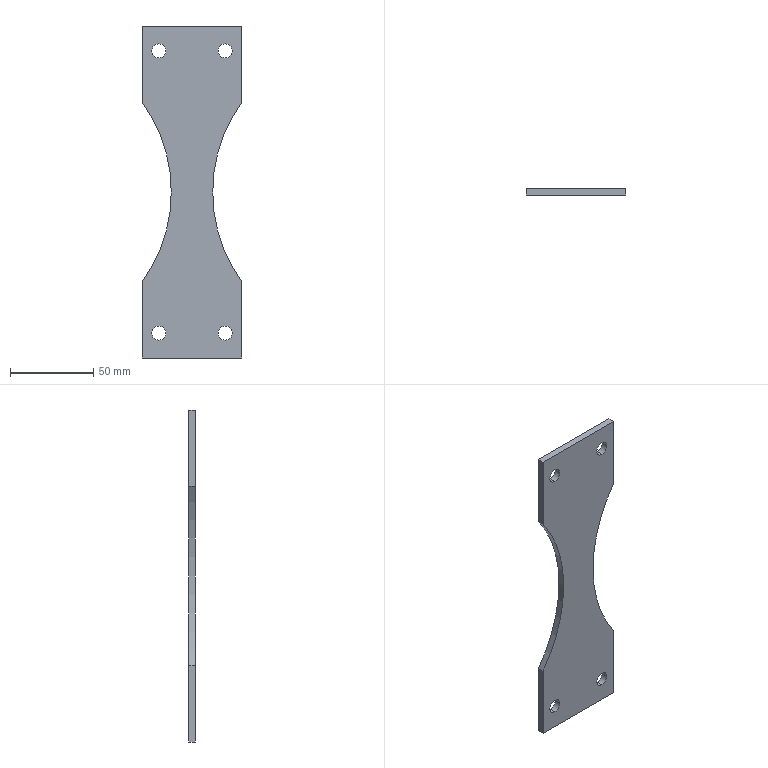Part | SolidWorks | features BaseBody 1 | 1 solid | 18 faces | box 60 x 4 x 200 mm | volume 36778 mm3 | cylinder 10 | plane 8 | commonest cylinder face diameters 8.5 x8 185 x2
STEP:
#1=CARTESIAN_POINT('',(671.946,-3637.973,1223.221));
#2=VERTEX_POINT('',#1);
#3=CARTESIAN_POINT('',(671.946,-3637.973,1214.721));
#4=VERTEX_POINT('',#3);
#5=CARTESIAN_POINT('',(671.946,-3637.973,1218.971));
#6=DIRECTION('',(0.,-1.,0.));
#7=DIRECTION('',(0.,0.,1.));
#8=AXIS2_PLACEMENT_3D('',#5,#6,#7);
#9=CIRCLE('',#8,4.25);
#10=EDGE_CURVE('',#2,#4,#9,.T.);
#11=ORIENTED_EDGE('',*,*,#10,.T.);
#12=CARTESIAN_POINT('',(671.946,-3633.973,1214.721));
#13=VERTEX_POINT('',#12);
#14=CARTESIAN_POINT('',(671.946,-3637.973,1214.721));
#15=DIRECTION('',(0.,1.,0.));
#16=VECTOR('',#15,1000.);
#17=LINE('',#14,#16);
#18=EDGE_CURVE('',#4,#13,#17,.T.);
#19=ORIENTED_EDGE('',*,*,#18,.T.);
#20=CARTESIAN_POINT('',(671.946,-3633.973,1223.221));
#21=VERTEX_POINT('',#20);
#22=CARTESIAN_POINT('',(671.946,-3633.973,1218.971));
#23=DIRECTION('',(0.,-1.,0.));
#24=DIRECTION('',(0.,0.,1.));
#25=AXIS2_PLACEMENT_3D('',#22,#23,#24);
#26=CIRCLE('',#25,4.25);
#27=EDGE_CURVE('',#21,#13,#26,.T.);
#28=ORIENTED_EDGE('',*,*,#27,.F.);
#29=CARTESIAN_POINT('',(671.946,-3637.973,1223.221));
#30=DIRECTION('',(0.,1.,0.));
#31=VECTOR('',#30,1000.);
#32=LINE('',#29,#31);
#33=EDGE_CURVE('',#2,#21,#32,.T.);
#34=ORIENTED_EDGE('',*,*,#33,.F.);
#35=EDGE_LOOP('',(#11,#19,#28,#34));
#36=FACE_OUTER_BOUND('',#35,.T.);
#37=CARTESIAN_POINT('',(671.946,-3637.973,1218.971));
#38=DIRECTION('',(0.,1.,0.));
#39=DIRECTION('',(0.,0.,1.));
#40=AXIS2_PLACEMENT_3D('',#37,#38,#39);
#41=CYLINDRICAL_SURFACE('',#40,4.25);
#42=ADVANCED_FACE('',(#36),#41,.F.);
#43=CARTESIAN_POINT('',(671.946,-3637.973,1393.221));
#44=VERTEX_POINT('',#43);
#45=CARTESIAN_POINT('',(671.946,-3637.973,1384.721));
#46=VERTEX_POINT('',#45);
#47=CARTESIAN_POINT('',(671.946,-3637.973,1388.971));
#48=DIRECTION('',(0.,-1.,0.));
#49=DIRECTION('',(0.,0.,1.));
#50=AXIS2_PLACEMENT_3D('',#47,#48,#49);
#51=CIRCLE('',#50,4.25);
#52=EDGE_CURVE('',#44,#46,#51,.T.);
#53=ORIENTED_EDGE('',*,*,#52,.T.);
#54=CARTESIAN_POINT('',(671.946,-3633.973,1384.721));
#55=VERTEX_POINT('',#54);
#56=CARTESIAN_POINT('',(671.946,-3637.973,1384.721));
#57=DIRECTION('',(0.,1.,0.));
#58=VECTOR('',#57,1000.);
#59=LINE('',#56,#58);
#60=EDGE_CURVE('',#46,#55,#59,.T.);
#61=ORIENTED_EDGE('',*,*,#60,.T.);
#62=CARTESIAN_POINT('',(671.946,-3633.973,1393.221));
#63=VERTEX_POINT('',#62);
#64=CARTESIAN_POINT('',(671.946,-3633.973,1388.971));
#65=DIRECTION('',(0.,-1.,0.));
#66=DIRECTION('',(0.,0.,1.));
#67=AXIS2_PLACEMENT_3D('',#64,#65,#66);
#68=CIRCLE('',#67,4.25);
#69=EDGE_CURVE('',#63,#55,#68,.T.);
#70=ORIENTED_EDGE('',*,*,#69,.F.);
#71=CARTESIAN_POINT('',(671.946,-3637.973,1393.221));
#72=DIRECTION('',(0.,1.,0.));
#73=VECTOR('',#72,1000.);
#74=LINE('',#71,#73);
#75=EDGE_CURVE('',#44,#63,#74,.T.);
#76=ORIENTED_EDGE('',*,*,#75,.F.);
#77=EDGE_LOOP('',(#53,#61,#70,#76));
#78=FACE_OUTER_BOUND('',#77,.T.);
#79=CARTESIAN_POINT('',(671.946,-3637.973,1388.971));
#80=DIRECTION('',(0.,1.,0.));
#81=DIRECTION('',(0.,0.,1.));
#82=AXIS2_PLACEMENT_3D('',#79,#80,#81);
#83=CYLINDRICAL_SURFACE('',#82,4.25);
#84=ADVANCED_FACE('',(#78),#83,.F.);
#85=CARTESIAN_POINT('',(631.946,-3637.973,1393.221));
#86=VERTEX_POINT('',#85);
#87=CARTESIAN_POINT('',(631.946,-3637.973,1384.721));
#88=VERTEX_POINT('',#87);
#89=CARTESIAN_POINT('',(631.946,-3637.973,1388.971));
#90=DIRECTION('',(0.,-1.,0.));
#91=DIRECTION('',(0.,0.,1.));
#92=AXIS2_PLACEMENT_3D('',#89,#90,#91);
#93=CIRCLE('',#92,4.25);
#94=EDGE_CURVE('',#86,#88,#93,.T.);
#95=ORIENTED_EDGE('',*,*,#94,.T.);
#96=CARTESIAN_POINT('',(631.946,-3633.973,1384.721));
#97=VERTEX_POINT('',#96);
#98=CARTESIAN_POINT('',(631.946,-3637.973,1384.721));
#99=DIRECTION('',(0.,1.,0.));
#100=VECTOR('',#99,1000.);
#101=LINE('',#98,#100);
#102=EDGE_CURVE('',#88,#97,#101,.T.);
#103=ORIENTED_EDGE('',*,*,#102,.T.);
#104=CARTESIAN_POINT('',(631.946,-3633.973,1393.221));
#105=VERTEX_POINT('',#104);
#106=CARTESIAN_POINT('',(631.946,-3633.973,1388.971));
#107=DIRECTION('',(0.,-1.,0.));
#108=DIRECTION('',(0.,0.,1.));
#109=AXIS2_PLACEMENT_3D('',#106,#107,#108);
#110=CIRCLE('',#109,4.25);
#111=EDGE_CURVE('',#105,#97,#110,.T.);
#112=ORIENTED_EDGE('',*,*,#111,.F.);
#113=CARTESIAN_POINT('',(631.946,-3637.973,1393.221));
#114=DIRECTION('',(0.,1.,0.));
#115=VECTOR('',#114,1000.);
#116=LINE('',#113,#115);
#117=EDGE_CURVE('',#86,#105,#116,.T.);
#118=ORIENTED_EDGE('',*,*,#117,.F.);
#119=EDGE_LOOP('',(#95,#103,#112,#118));
#120=FACE_OUTER_BOUND('',#119,.T.);
#121=CARTESIAN_POINT('',(631.946,-3637.973,1388.971));
#122=DIRECTION('',(0.,1.,0.));
#123=DIRECTION('',(0.,0.,1.));
#124=AXIS2_PLACEMENT_3D('',#121,#122,#123);
#125=CYLINDRICAL_SURFACE('',#124,4.25);
#126=ADVANCED_FACE('',(#120),#125,.F.);
#127=CARTESIAN_POINT('',(631.946,-3637.973,1223.221));
#128=VERTEX_POINT('',#127);
#129=CARTESIAN_POINT('',(631.946,-3637.973,1214.721));
#130=VERTEX_POINT('',#129);
#131=CARTESIAN_POINT('',(631.946,-3637.973,1218.971));
#132=DIRECTION('',(0.,-1.,0.));
#133=DIRECTION('',(0.,0.,1.));
#134=AXIS2_PLACEMENT_3D('',#131,#132,#133);
#135=CIRCLE('',#134,4.25);
#136=EDGE_CURVE('',#128,#130,#135,.T.);
#137=ORIENTED_EDGE('',*,*,#136,.T.);
#138=CARTESIAN_POINT('',(631.946,-3633.973,1214.721));
#139=VERTEX_POINT('',#138);
#140=CARTESIAN_POINT('',(631.946,-3637.973,1214.721));
#141=DIRECTION('',(0.,1.,0.));
#142=VECTOR('',#141,1000.);
#143=LINE('',#140,#142);
#144=EDGE_CURVE('',#130,#139,#143,.T.);
#145=ORIENTED_EDGE('',*,*,#144,.T.);
#146=CARTESIAN_POINT('',(631.946,-3633.973,1223.221));
#147=VERTEX_POINT('',#146);
#148=CARTESIAN_POINT('',(631.946,-3633.973,1218.971));
#149=DIRECTION('',(0.,-1.,0.));
#150=DIRECTION('',(0.,0.,1.));
#151=AXIS2_PLACEMENT_3D('',#148,#149,#150);
#152=CIRCLE('',#151,4.25);
#153=EDGE_CURVE('',#147,#139,#152,.T.);
#154=ORIENTED_EDGE('',*,*,#153,.F.);
#155=CARTESIAN_POINT('',(631.946,-3637.973,1223.221));
#156=DIRECTION('',(0.,1.,0.));
#157=VECTOR('',#156,1000.);
#158=LINE('',#155,#157);
#159=EDGE_CURVE('',#128,#147,#158,.T.);
#160=ORIENTED_EDGE('',*,*,#159,.F.);
#161=EDGE_LOOP('',(#137,#145,#154,#160));
#162=FACE_OUTER_BOUND('',#161,.T.);
#163=CARTESIAN_POINT('',(631.946,-3637.973,1218.971));
#164=DIRECTION('',(0.,1.,0.));
#165=DIRECTION('',(0.,0.,1.));
#166=AXIS2_PLACEMENT_3D('',#163,#164,#165);
#167=CYLINDRICAL_SURFACE('',#166,4.25);
#168=ADVANCED_FACE('',(#162),#167,.F.);
#169=CARTESIAN_POINT('',(681.946,-3633.973,1403.971));
#170=VERTEX_POINT('',#169);
#171=CARTESIAN_POINT('',(681.946,-3633.973,1358.112));
#172=VERTEX_POINT('',#171);
#173=CARTESIAN_POINT('',(681.946,-3633.973,1303.971));
#174=DIRECTION('',(0.,0.,-1.));
#175=VECTOR('',#174,1000.);
#176=LINE('',#173,#175);
#177=EDGE_CURVE('',#170,#172,#176,.T.);
#178=ORIENTED_EDGE('',*,*,#177,.T.);
#179=CARTESIAN_POINT('',(681.946,-3633.973,1249.83));
#180=VERTEX_POINT('',#179);
#181=CARTESIAN_POINT('',(756.946,-3633.973,1303.971));
#182=DIRECTION('',(0.,-1.,0.));
#183=DIRECTION('',(0.,0.,1.));
#184=AXIS2_PLACEMENT_3D('',#181,#182,#183);
#185=CIRCLE('',#184,92.5);
#186=EDGE_CURVE('',#172,#180,#185,.T.);
#187=ORIENTED_EDGE('',*,*,#186,.T.);
#188=CARTESIAN_POINT('',(681.946,-3633.973,1203.971));
#189=VERTEX_POINT('',#188);
#190=CARTESIAN_POINT('',(681.946,-3633.973,1303.971));
#191=DIRECTION('',(0.,0.,-1.));
#192=VECTOR('',#191,1000.);
#193=LINE('',#190,#192);
#194=EDGE_CURVE('',#180,#189,#193,.T.);
#195=ORIENTED_EDGE('',*,*,#194,.T.);
#196=CARTESIAN_POINT('',(621.946,-3633.973,1203.971));
#197=VERTEX_POINT('',#196);
#198=CARTESIAN_POINT('',(651.946,-3633.973,1203.971));
#199=DIRECTION('',(-1.,0.,0.));
#200=VECTOR('',#199,1000.);
#201=LINE('',#198,#200);
#202=EDGE_CURVE('',#189,#197,#201,.T.);
#203=ORIENTED_EDGE('',*,*,#202,.T.);
#204=CARTESIAN_POINT('',(621.946,-3633.973,1249.83));
#205=VERTEX_POINT('',#204);
#206=CARTESIAN_POINT('',(621.946,-3633.973,1303.971));
#207=DIRECTION('',(0.,0.,1.));
#208=VECTOR('',#207,1000.);
#209=LINE('',#206,#208);
#210=EDGE_CURVE('',#197,#205,#209,.T.);
#211=ORIENTED_EDGE('',*,*,#210,.T.);
#212=CARTESIAN_POINT('',(621.946,-3633.973,1358.112));
#213=VERTEX_POINT('',#212);
#214=CARTESIAN_POINT('',(546.946,-3633.973,1303.971));
#215=DIRECTION('',(0.,-1.,0.));
#216=DIRECTION('',(0.,0.,1.));
#217=AXIS2_PLACEMENT_3D('',#214,#215,#216);
#218=CIRCLE('',#217,92.5);
#219=EDGE_CURVE('',#205,#213,#218,.T.);
#220=ORIENTED_EDGE('',*,*,#219,.T.);
#221=CARTESIAN_POINT('',(621.946,-3633.973,1403.971));
#222=VERTEX_POINT('',#221);
#223=CARTESIAN_POINT('',(621.946,-3633.973,1303.971));
#224=DIRECTION('',(0.,0.,1.));
#225=VECTOR('',#224,1000.);
#226=LINE('',#223,#225);
#227=EDGE_CURVE('',#213,#222,#226,.T.);
#228=ORIENTED_EDGE('',*,*,#227,.T.);
#229=CARTESIAN_POINT('',(651.946,-3633.973,1403.971));
#230=DIRECTION('',(1.,0.,0.));
#231=VECTOR('',#230,1000.);
#232=LINE('',#229,#231);
#233=EDGE_CURVE('',#222,#170,#232,.T.);
#234=ORIENTED_EDGE('',*,*,#233,.T.);
#235=EDGE_LOOP('',(#178,#187,#195,#203,#211,#220,#228,#234));
#236=FACE_OUTER_BOUND('',#235,.T.);
#237=ORIENTED_EDGE('',*,*,#27,.T.);
#238=CARTESIAN_POINT('',(671.946,-3633.973,1218.971));
#239=DIRECTION('',(0.,-1.,0.));
#240=DIRECTION('',(0.,0.,1.));
#241=AXIS2_PLACEMENT_3D('',#238,#239,#240);
#242=CIRCLE('',#241,4.25);
#243=EDGE_CURVE('',#13,#21,#242,.T.);
#244=ORIENTED_EDGE('',*,*,#243,.T.);
#245=EDGE_LOOP('',(#237,#244));
#246=FACE_BOUND('',#245,.T.);
#247=ORIENTED_EDGE('',*,*,#69,.T.);
#248=CARTESIAN_POINT('',(671.946,-3633.973,1388.971));
#249=DIRECTION('',(0.,-1.,0.));
#250=DIRECTION('',(0.,0.,1.));
#251=AXIS2_PLACEMENT_3D('',#248,#249,#250);
#252=CIRCLE('',#251,4.25);
#253=EDGE_CURVE('',#55,#63,#252,.T.);
#254=ORIENTED_EDGE('',*,*,#253,.T.);
#255=EDGE_LOOP('',(#247,#254));
#256=FACE_BOUND('',#255,.T.);
#257=ORIENTED_EDGE('',*,*,#111,.T.);
#258=CARTESIAN_POINT('',(631.946,-3633.973,1388.971));
#259=DIRECTION('',(0.,-1.,0.));
#260=DIRECTION('',(0.,0.,1.));
#261=AXIS2_PLACEMENT_3D('',#258,#259,#260);
#262=CIRCLE('',#261,4.25);
#263=EDGE_CURVE('',#97,#105,#262,.T.);
#264=ORIENTED_EDGE('',*,*,#263,.T.);
#265=EDGE_LOOP('',(#257,#264));
#266=FACE_BOUND('',#265,.T.);
#267=ORIENTED_EDGE('',*,*,#153,.T.);
#268=CARTESIAN_POINT('',(631.946,-3633.973,1218.971));
#269=DIRECTION('',(0.,-1.,0.));
#270=DIRECTION('',(0.,0.,1.));
#271=AXIS2_PLACEMENT_3D('',#268,#269,#270);
#272=CIRCLE('',#271,4.25);
#273=EDGE_CURVE('',#139,#147,#272,.T.);
#274=ORIENTED_EDGE('',*,*,#273,.T.);
#275=EDGE_LOOP('',(#267,#274));
#276=FACE_BOUND('',#275,.T.);
#277=CARTESIAN_POINT('',(651.946,-3633.973,1303.971));
#278=DIRECTION('',(0.,1.,0.));
#279=DIRECTION('',(0.,0.,1.));
#280=AXIS2_PLACEMENT_3D('',#277,#278,#279);
#281=PLANE('',#280);
#282=ADVANCED_FACE('',(#236,#246,#256,#266,#276),#281,.T.);
#283=ORIENTED_EDGE('',*,*,#186,.F.);
#284=CARTESIAN_POINT('',(681.946,-3637.973,1358.112));
#285=VERTEX_POINT('',#284);
#286=CARTESIAN_POINT('',(681.946,-3633.973,1358.112));
#287=DIRECTION('',(0.,-1.,0.));
#288=VECTOR('',#287,1000.);
#289=LINE('',#286,#288);
#290=EDGE_CURVE('',#172,#285,#289,.T.);
#291=ORIENTED_EDGE('',*,*,#290,.T.);
#292=CARTESIAN_POINT('',(681.946,-3637.973,1249.83));
#293=VERTEX_POINT('',#292);
#294=CARTESIAN_POINT('',(756.946,-3637.973,1303.971));
#295=DIRECTION('',(0.,-1.,0.));
#296=DIRECTION('',(0.,0.,1.));
#297=AXIS2_PLACEMENT_3D('',#294,#295,#296);
#298=CIRCLE('',#297,92.5);
#299=EDGE_CURVE('',#285,#293,#298,.T.);
#300=ORIENTED_EDGE('',*,*,#299,.T.);
#301=CARTESIAN_POINT('',(681.946,-3633.973,1249.83));
#302=DIRECTION('',(0.,1.,0.));
#303=VECTOR('',#302,1000.);
#304=LINE('',#301,#303);
#305=EDGE_CURVE('',#293,#180,#304,.T.);
#306=ORIENTED_EDGE('',*,*,#305,.T.);
#307=EDGE_LOOP('',(#283,#291,#300,#306));
#308=FACE_OUTER_BOUND('',#307,.T.);
#309=CARTESIAN_POINT('',(756.946,-3637.973,1303.971));
#310=DIRECTION('',(0.,1.,0.));
#311=DIRECTION('',(0.,0.,1.));
#312=AXIS2_PLACEMENT_3D('',#309,#310,#311);
#313=CYLINDRICAL_SURFACE('',#312,92.5);
#314=ADVANCED_FACE('',(#308),#313,.F.);
#315=ORIENTED_EDGE('',*,*,#177,.F.);
#316=CARTESIAN_POINT('',(681.946,-3637.973,1403.971));
#317=VERTEX_POINT('',#316);
#318=CARTESIAN_POINT('',(681.946,-3633.973,1403.971));
#319=DIRECTION('',(0.,-1.,0.));
#320=VECTOR('',#319,1000.);
#321=LINE('',#318,#320);
#322=EDGE_CURVE('',#170,#317,#321,.T.);
#323=ORIENTED_EDGE('',*,*,#322,.T.);
#324=CARTESIAN_POINT('',(681.946,-3637.973,1358.112));
#325=DIRECTION('',(0.,0.,-1.));
#326=VECTOR('',#325,1000.);
#327=LINE('',#324,#326);
#328=EDGE_CURVE('',#317,#285,#327,.T.);
#329=ORIENTED_EDGE('',*,*,#328,.T.);
#330=ORIENTED_EDGE('',*,*,#290,.F.);
#331=EDGE_LOOP('',(#315,#323,#329,#330));
#332=FACE_OUTER_BOUND('',#331,.T.);
#333=CARTESIAN_POINT('',(681.946,-3633.973,1358.112));
#334=DIRECTION('',(1.,0.,0.));
#335=DIRECTION('',(0.,0.,-1.));
#336=AXIS2_PLACEMENT_3D('',#333,#334,#335);
#337=PLANE('',#336);
#338=ADVANCED_FACE('',(#332),#337,.T.);
#339=ORIENTED_EDGE('',*,*,#233,.F.);
#340=CARTESIAN_POINT('',(621.946,-3637.973,1403.971));
#341=VERTEX_POINT('',#340);
#342=CARTESIAN_POINT('',(621.946,-3633.973,1403.971));
#343=DIRECTION('',(0.,-1.,0.));
#344=VECTOR('',#343,1000.);
#345=LINE('',#342,#344);
#346=EDGE_CURVE('',#222,#341,#345,.T.);
#347=ORIENTED_EDGE('',*,*,#346,.T.);
#348=CARTESIAN_POINT('',(681.946,-3637.973,1403.971));
#349=DIRECTION('',(1.,0.,0.));
#350=VECTOR('',#349,1000.);
#351=LINE('',#348,#350);
#352=EDGE_CURVE('',#341,#317,#351,.T.);
#353=ORIENTED_EDGE('',*,*,#352,.T.);
#354=ORIENTED_EDGE('',*,*,#322,.F.);
#355=EDGE_LOOP('',(#339,#347,#353,#354));
#356=FACE_OUTER_BOUND('',#355,.T.);
#357=CARTESIAN_POINT('',(681.946,-3633.973,1403.971));
#358=DIRECTION('',(0.,0.,1.));
#359=DIRECTION('',(1.,0.,0.));
#360=AXIS2_PLACEMENT_3D('',#357,#358,#359);
#361=PLANE('',#360);
#362=ADVANCED_FACE('',(#356),#361,.T.);
#363=ORIENTED_EDGE('',*,*,#227,.F.);
#364=CARTESIAN_POINT('',(621.946,-3637.973,1358.112));
#365=VERTEX_POINT('',#364);
#366=CARTESIAN_POINT('',(621.946,-3633.973,1358.112));
#367=DIRECTION('',(0.,-1.,0.));
#368=VECTOR('',#367,1000.);
#369=LINE('',#366,#368);
#370=EDGE_CURVE('',#213,#365,#369,.T.);
#371=ORIENTED_EDGE('',*,*,#370,.T.);
#372=CARTESIAN_POINT('',(621.946,-3637.973,1403.971));
#373=DIRECTION('',(0.,0.,1.));
#374=VECTOR('',#373,1000.);
#375=LINE('',#372,#374);
#376=EDGE_CURVE('',#365,#341,#375,.T.);
#377=ORIENTED_EDGE('',*,*,#376,.T.);
#378=ORIENTED_EDGE('',*,*,#346,.F.);
#379=EDGE_LOOP('',(#363,#371,#377,#378));
#380=FACE_OUTER_BOUND('',#379,.T.);
#381=CARTESIAN_POINT('',(621.946,-3633.973,1403.971));
#382=DIRECTION('',(-1.,0.,0.));
#383=DIRECTION('',(0.,0.,1.));
#384=AXIS2_PLACEMENT_3D('',#381,#382,#383);
#385=PLANE('',#384);
#386=ADVANCED_FACE('',(#380),#385,.T.);
#387=ORIENTED_EDGE('',*,*,#219,.F.);
#388=CARTESIAN_POINT('',(621.946,-3637.973,1249.83));
#389=VERTEX_POINT('',#388);
#390=CARTESIAN_POINT('',(621.946,-3633.973,1249.83));
#391=DIRECTION('',(0.,-1.,0.));
#392=VECTOR('',#391,1000.);
#393=LINE('',#390,#392);
#394=EDGE_CURVE('',#205,#389,#393,.T.);
#395=ORIENTED_EDGE('',*,*,#394,.T.);
#396=CARTESIAN_POINT('',(546.946,-3637.973,1303.971));
#397=DIRECTION('',(0.,-1.,0.));
#398=DIRECTION('',(0.,0.,1.));
#399=AXIS2_PLACEMENT_3D('',#396,#397,#398);
#400=CIRCLE('',#399,92.5);
#401=EDGE_CURVE('',#389,#365,#400,.T.);
#402=ORIENTED_EDGE('',*,*,#401,.T.);
#403=ORIENTED_EDGE('',*,*,#370,.F.);
#404=EDGE_LOOP('',(#387,#395,#402,#403));
#405=FACE_OUTER_BOUND('',#404,.T.);
#406=CARTESIAN_POINT('',(546.946,-3637.973,1303.971));
#407=DIRECTION('',(0.,1.,0.));
#408=DIRECTION('',(0.,0.,1.));
#409=AXIS2_PLACEMENT_3D('',#406,#407,#408);
#410=CYLINDRICAL_SURFACE('',#409,92.5);
#411=ADVANCED_FACE('',(#405),#410,.F.);
#412=ORIENTED_EDGE('',*,*,#210,.F.);
#413=CARTESIAN_POINT('',(621.946,-3637.973,1203.971));
#414=VERTEX_POINT('',#413);
#415=CARTESIAN_POINT('',(621.946,-3633.973,1203.971));
#416=DIRECTION('',(0.,-1.,0.));
#417=VECTOR('',#416,1000.);
#418=LINE('',#415,#417);
#419=EDGE_CURVE('',#197,#414,#418,.T.);
#420=ORIENTED_EDGE('',*,*,#419,.T.);
#421=CARTESIAN_POINT('',(621.946,-3637.973,1249.83));
#422=DIRECTION('',(0.,0.,1.));
#423=VECTOR('',#422,1000.);
#424=LINE('',#421,#423);
#425=EDGE_CURVE('',#414,#389,#424,.T.);
#426=ORIENTED_EDGE('',*,*,#425,.T.);
#427=ORIENTED_EDGE('',*,*,#394,.F.);
#428=EDGE_LOOP('',(#412,#420,#426,#427));
#429=FACE_OUTER_BOUND('',#428,.T.);
#430=CARTESIAN_POINT('',(621.946,-3633.973,1249.83));
#431=DIRECTION('',(-1.,0.,0.));
#432=DIRECTION('',(0.,0.,1.));
#433=AXIS2_PLACEMENT_3D('',#430,#431,#432);
#434=PLANE('',#433);
#435=ADVANCED_FACE('',(#429),#434,.T.);
#436=ORIENTED_EDGE('',*,*,#202,.F.);
#437=CARTESIAN_POINT('',(681.946,-3637.973,1203.971));
#438=VERTEX_POINT('',#437);
#439=CARTESIAN_POINT('',(681.946,-3633.973,1203.971));
#440=DIRECTION('',(0.,-1.,0.));
#441=VECTOR('',#440,1000.);
#442=LINE('',#439,#441);
#443=EDGE_CURVE('',#189,#438,#442,.T.);
#444=ORIENTED_EDGE('',*,*,#443,.T.);
#445=CARTESIAN_POINT('',(621.946,-3637.973,1203.971));
#446=DIRECTION('',(-1.,0.,0.));
#447=VECTOR('',#446,1000.);
#448=LINE('',#445,#447);
#449=EDGE_CURVE('',#438,#414,#448,.T.);
#450=ORIENTED_EDGE('',*,*,#449,.T.);
#451=ORIENTED_EDGE('',*,*,#419,.F.);
#452=EDGE_LOOP('',(#436,#444,#450,#451));
#453=FACE_OUTER_BOUND('',#452,.T.);
#454=CARTESIAN_POINT('',(621.946,-3633.973,1203.971));
#455=DIRECTION('',(0.,0.,-1.));
#456=DIRECTION('',(-1.,0.,0.));
#457=AXIS2_PLACEMENT_3D('',#454,#455,#456);
#458=PLANE('',#457);
#459=ADVANCED_FACE('',(#453),#458,.T.);
#460=ORIENTED_EDGE('',*,*,#194,.F.);
#461=ORIENTED_EDGE('',*,*,#305,.F.);
#462=CARTESIAN_POINT('',(681.946,-3637.973,1203.971));
#463=DIRECTION('',(0.,0.,-1.));
#464=VECTOR('',#463,1000.);
#465=LINE('',#462,#464);
#466=EDGE_CURVE('',#293,#438,#465,.T.);
#467=ORIENTED_EDGE('',*,*,#466,.T.);
#468=ORIENTED_EDGE('',*,*,#443,.F.);
#469=EDGE_LOOP('',(#460,#461,#467,#468));
#470=FACE_OUTER_BOUND('',#469,.T.);
#471=CARTESIAN_POINT('',(681.946,-3633.973,1203.971));
#472=DIRECTION('',(1.,0.,0.));
#473=DIRECTION('',(0.,0.,-1.));
#474=AXIS2_PLACEMENT_3D('',#471,#472,#473);
#475=PLANE('',#474);
#476=ADVANCED_FACE('',(#470),#475,.T.);
#477=ORIENTED_EDGE('',*,*,#18,.F.);
#478=CARTESIAN_POINT('',(671.946,-3637.973,1218.971));
#479=DIRECTION('',(0.,-1.,0.));
#480=DIRECTION('',(0.,0.,1.));
#481=AXIS2_PLACEMENT_3D('',#478,#479,#480);
#482=CIRCLE('',#481,4.25);
#483=EDGE_CURVE('',#4,#2,#482,.T.);
#484=ORIENTED_EDGE('',*,*,#483,.T.);
#485=ORIENTED_EDGE('',*,*,#33,.T.);
#486=ORIENTED_EDGE('',*,*,#243,.F.);
#487=EDGE_LOOP('',(#477,#484,#485,#486));
#488=FACE_OUTER_BOUND('',#487,.T.);
#489=CARTESIAN_POINT('',(671.946,-3637.973,1218.971));
#490=DIRECTION('',(0.,1.,0.));
#491=DIRECTION('',(0.,0.,1.));
#492=AXIS2_PLACEMENT_3D('',#489,#490,#491);
#493=CYLINDRICAL_SURFACE('',#492,4.25);
#494=ADVANCED_FACE('',(#488),#493,.F.);
#495=ORIENTED_EDGE('',*,*,#60,.F.);
#496=CARTESIAN_POINT('',(671.946,-3637.973,1388.971));
#497=DIRECTION('',(0.,-1.,0.));
#498=DIRECTION('',(0.,0.,1.));
#499=AXIS2_PLACEMENT_3D('',#496,#497,#498);
#500=CIRCLE('',#499,4.25);
#501=EDGE_CURVE('',#46,#44,#500,.T.);
#502=ORIENTED_EDGE('',*,*,#501,.T.);
#503=ORIENTED_EDGE('',*,*,#75,.T.);
#504=ORIENTED_EDGE('',*,*,#253,.F.);
#505=EDGE_LOOP('',(#495,#502,#503,#504));
#506=FACE_OUTER_BOUND('',#505,.T.);
#507=CARTESIAN_POINT('',(671.946,-3637.973,1388.971));
#508=DIRECTION('',(0.,1.,0.));
#509=DIRECTION('',(0.,0.,1.));
#510=AXIS2_PLACEMENT_3D('',#507,#508,#509);
#511=CYLINDRICAL_SURFACE('',#510,4.25);
#512=ADVANCED_FACE('',(#506),#511,.F.);
#513=ORIENTED_EDGE('',*,*,#102,.F.);
#514=CARTESIAN_POINT('',(631.946,-3637.973,1388.971));
#515=DIRECTION('',(0.,-1.,0.));
#516=DIRECTION('',(0.,0.,1.));
#517=AXIS2_PLACEMENT_3D('',#514,#515,#516);
#518=CIRCLE('',#517,4.25);
#519=EDGE_CURVE('',#88,#86,#518,.T.);
#520=ORIENTED_EDGE('',*,*,#519,.T.);
#521=ORIENTED_EDGE('',*,*,#117,.T.);
#522=ORIENTED_EDGE('',*,*,#263,.F.);
#523=EDGE_LOOP('',(#513,#520,#521,#522));
#524=FACE_OUTER_BOUND('',#523,.T.);
#525=CARTESIAN_POINT('',(631.946,-3637.973,1388.971));
#526=DIRECTION('',(0.,1.,0.));
#527=DIRECTION('',(0.,0.,1.));
#528=AXIS2_PLACEMENT_3D('',#525,#526,#527);
#529=CYLINDRICAL_SURFACE('',#528,4.25);
#530=ADVANCED_FACE('',(#524),#529,.F.);
#531=ORIENTED_EDGE('',*,*,#144,.F.);
#532=CARTESIAN_POINT('',(631.946,-3637.973,1218.971));
#533=DIRECTION('',(0.,-1.,0.));
#534=DIRECTION('',(0.,0.,1.));
#535=AXIS2_PLACEMENT_3D('',#532,#533,#534);
#536=CIRCLE('',#535,4.25);
#537=EDGE_CURVE('',#130,#128,#536,.T.);
#538=ORIENTED_EDGE('',*,*,#537,.T.);
#539=ORIENTED_EDGE('',*,*,#159,.T.);
#540=ORIENTED_EDGE('',*,*,#273,.F.);
#541=EDGE_LOOP('',(#531,#538,#539,#540));
#542=FACE_OUTER_BOUND('',#541,.T.);
#543=CARTESIAN_POINT('',(631.946,-3637.973,1218.971));
#544=DIRECTION('',(0.,1.,0.));
#545=DIRECTION('',(0.,0.,1.));
#546=AXIS2_PLACEMENT_3D('',#543,#544,#545);
#547=CYLINDRICAL_SURFACE('',#546,4.25);
#548=ADVANCED_FACE('',(#542),#547,.F.);
#549=ORIENTED_EDGE('',*,*,#328,.F.);
#550=ORIENTED_EDGE('',*,*,#352,.F.);
#551=ORIENTED_EDGE('',*,*,#376,.F.);
#552=ORIENTED_EDGE('',*,*,#401,.F.);
#553=ORIENTED_EDGE('',*,*,#425,.F.);
#554=ORIENTED_EDGE('',*,*,#449,.F.);
#555=ORIENTED_EDGE('',*,*,#466,.F.);
#556=ORIENTED_EDGE('',*,*,#299,.F.);
#557=EDGE_LOOP('',(#549,#550,#551,#552,#553,#554,#555,#556));
#558=FACE_OUTER_BOUND('',#557,.T.);
#559=ORIENTED_EDGE('',*,*,#10,.F.);
#560=ORIENTED_EDGE('',*,*,#483,.F.);
#561=EDGE_LOOP('',(#559,#560));
#562=FACE_BOUND('',#561,.T.);
#563=ORIENTED_EDGE('',*,*,#52,.F.);
#564=ORIENTED_EDGE('',*,*,#501,.F.);
#565=EDGE_LOOP('',(#563,#564));
#566=FACE_BOUND('',#565,.T.);
#567=ORIENTED_EDGE('',*,*,#94,.F.);
#568=ORIENTED_EDGE('',*,*,#519,.F.);
#569=EDGE_LOOP('',(#567,#568));
#570=FACE_BOUND('',#569,.T.);
#571=ORIENTED_EDGE('',*,*,#136,.F.);
#572=ORIENTED_EDGE('',*,*,#537,.F.);
#573=EDGE_LOOP('',(#571,#572));
#574=FACE_BOUND('',#573,.T.);
#575=CARTESIAN_POINT('',(651.946,-3637.973,1303.971));
#576=DIRECTION('',(0.,1.,0.));
#577=DIRECTION('',(0.,0.,1.));
#578=AXIS2_PLACEMENT_3D('',#575,#576,#577);
#579=PLANE('',#578);
#580=ADVANCED_FACE('',(#558,#562,#566,#570,#574),#579,.F.);
#581=CLOSED_SHELL('',(#42,#84,#126,#168,#282,#314,#338,#362,#386,#411,#435,#459,#476,#494,#512,#530,#548,#580));
#582=MANIFOLD_SOLID_BREP('',#581);
#583=CARTESIAN_POINT('',(0.,0.,0.));
#584=DIRECTION('',(0.,0.,1.));
#585=DIRECTION('',(1.,0.,0.));
#586=AXIS2_PLACEMENT_3D('',#583,#584,#585);
#587=(LENGTH_UNIT()NAMED_UNIT(*)SI_UNIT(.MILLI.,.METRE.));
#588=UNCERTAINTY_MEASURE_WITH_UNIT(LENGTH_MEASURE(0.00001),#587,'','');
#589=(NAMED_UNIT(*)PLANE_ANGLE_UNIT()SI_UNIT($,.RADIAN.));
#590=(NAMED_UNIT(*)SI_UNIT($,.STERADIAN.)SOLID_ANGLE_UNIT());
#591=(GEOMETRIC_REPRESENTATION_CONTEXT(3)GLOBAL_UNCERTAINTY_ASSIGNED_CONTEXT((#588))GLOBAL_UNIT_ASSIGNED_CONTEXT((#587,#589,#590))REPRESENTATION_CONTEXT('',''));
#592=ADVANCED_BREP_SHAPE_REPRESENTATION('',(#582,#586),#591);